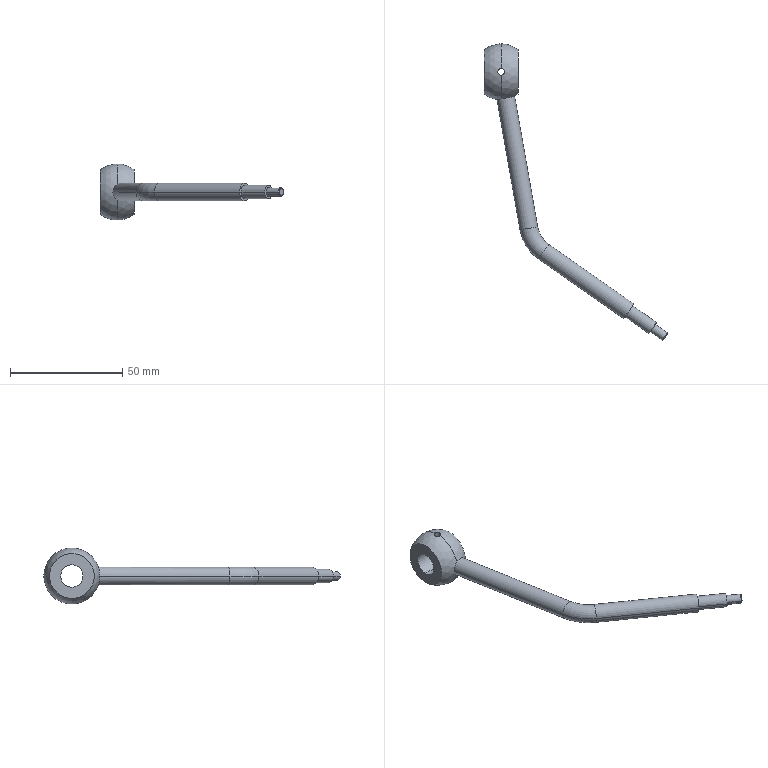Part | SolidWorks | features ICE 4, Revolution 1, StudWizard 1, Sweep 1, SweepCut 1 | 1 solid | 25 faces | box 81.686 x 132.115 x 24.819 mm | volume 11563 mm3 | cylinder 14 | plane 5 | torus 2 | cone 2 | sphere 2 | commonest cylinder face diameters 3 x4 8 x4 4 x2 6 x2 10 x2
STEP:
#1=CARTESIAN_POINT('',(8.368,-70.49,0.));
#2=VERTEX_POINT('',#1);
#3=CARTESIAN_POINT('',(16.246,-69.101,0.));
#4=VERTEX_POINT('',#3);
#5=CARTESIAN_POINT('',(12.307,-69.796,0.));
#6=DIRECTION('',(-0.1736,0.9848,0.));
#7=DIRECTION('',(-0.9848,-0.1736,0.));
#8=AXIS2_PLACEMENT_3D('',#5,#6,#7);
#9=CIRCLE('',#8,4.);
#10=EDGE_CURVE('',#2,#4,#9,.T.);
#11=ORIENTED_EDGE('',*,*,#10,.F.);
#12=CARTESIAN_POINT('',(16.592,-83.401,0.));
#13=VERTEX_POINT('',#12);
#14=CARTESIAN_POINT('',(28.064,-67.017,0.));
#15=DIRECTION('',(0.,0.,1.));
#16=DIRECTION('',(1.,0.,0.));
#17=AXIS2_PLACEMENT_3D('',#14,#15,#16);
#18=CIRCLE('',#17,20.);
#19=EDGE_CURVE('',#2,#13,#18,.T.);
#20=ORIENTED_EDGE('',*,*,#19,.T.);
#21=CARTESIAN_POINT('',(21.181,-76.847,0.));
#22=VERTEX_POINT('',#21);
#23=CARTESIAN_POINT('',(18.887,-80.124,0.));
#24=DIRECTION('',(-0.8192,0.5736,0.));
#25=DIRECTION('',(-0.5736,-0.8192,0.));
#26=AXIS2_PLACEMENT_3D('',#23,#24,#25);
#27=CIRCLE('',#26,4.);
#28=EDGE_CURVE('',#13,#22,#27,.T.);
#29=ORIENTED_EDGE('',*,*,#28,.T.);
#30=CARTESIAN_POINT('',(28.064,-67.017,0.));
#31=DIRECTION('',(0.,0.,1.));
#32=DIRECTION('',(1.,0.,0.));
#33=AXIS2_PLACEMENT_3D('',#30,#31,#32);
#34=CIRCLE('',#33,12.);
#35=EDGE_CURVE('',#4,#22,#34,.T.);
#36=ORIENTED_EDGE('',*,*,#35,.F.);
#37=EDGE_LOOP('',(#11,#20,#29,#36));
#38=FACE_OUTER_BOUND('',#37,.T.);
#39=CARTESIAN_POINT('',(28.064,-67.017,0.));
#40=DIRECTION('',(0.,0.,1.));
#41=DIRECTION('',(1.,0.,0.));
#42=AXIS2_PLACEMENT_3D('',#39,#40,#41);
#43=TOROIDAL_SURFACE('',#42,16.,4.);
#44=ADVANCED_FACE('',(#38),#43,.T.);
#45=CARTESIAN_POINT('',(1.5,0.,-5.));
#46=VERTEX_POINT('',#45);
#47=CARTESIAN_POINT('',(-1.5,0.,-5.));
#48=VERTEX_POINT('',#47);
#49=CARTESIAN_POINT('',(1.5,0.,-5.));
#50=CARTESIAN_POINT('',(1.5,-0.1965,-5.));
#51=CARTESIAN_POINT('',(1.46,-0.3949,-4.988));
#52=CARTESIAN_POINT('',(1.348,-0.6661,-4.956));
#53=CARTESIAN_POINT('',(1.3,-0.7539,-4.944));
#54=CARTESIAN_POINT('',(1.192,-0.9162,-4.916));
#55=CARTESIAN_POINT('',(1.13,-0.9913,-4.901));
#56=CARTESIAN_POINT('',(0.9224,-1.199,-4.856));
#57=CARTESIAN_POINT('',(0.7589,-1.309,-4.826));
#58=CARTESIAN_POINT('',(0.4847,-1.423,-4.793));
#59=CARTESIAN_POINT('',(0.3909,-1.451,-4.785));
#60=CARTESIAN_POINT('',(0.1987,-1.49,-4.773));
#61=CARTESIAN_POINT('',(0.09898,-1.5,-4.77));
#62=CARTESIAN_POINT('',(-0.09875,-1.5,-4.77));
#63=CARTESIAN_POINT('',(-0.1965,-1.49,-4.773));
#64=CARTESIAN_POINT('',(-0.3898,-1.452,-4.785));
#65=CARTESIAN_POINT('',(-0.4854,-1.423,-4.793));
#66=CARTESIAN_POINT('',(-0.7564,-1.31,-4.826));
#67=CARTESIAN_POINT('',(-0.9227,-1.199,-4.856));
#68=CARTESIAN_POINT('',(-1.129,-0.9924,-4.901));
#69=CARTESIAN_POINT('',(-1.192,-0.9159,-4.916));
#70=CARTESIAN_POINT('',(-1.301,-0.7533,-4.944));
#71=CARTESIAN_POINT('',(-1.347,-0.6674,-4.956));
#72=CARTESIAN_POINT('',(-1.422,-0.4865,-4.977));
#73=CARTESIAN_POINT('',(-1.452,-0.3907,-4.986));
#74=CARTESIAN_POINT('',(-1.49,-0.1978,-4.997));
#75=CARTESIAN_POINT('',(-1.5,-0.0997,-5.));
#76=CARTESIAN_POINT('',(-1.5,0.,-5.));
#77=B_SPLINE_CURVE_WITH_KNOTS('',3,(#49,#50,#51,#52,#53,#54,#55,#56,#57,#58,#59,#60,#61,#62,#63,#64,#65,#66,#67,#68,#69,#70,#71,#72,#73,#74,#75,#76),.UNSPECIFIED.,.F.,.F.,(4,2,2,2,2,2,2,2,2,2,2,2,2,4),(0.004717,0.005306,0.005601,0.005896,0.006485,0.00678,0.007075,0.00737,0.007664,0.008254,0.008549,0.008843,0.009138,0.009433),.UNSPECIFIED.);
#78=EDGE_CURVE('',#46,#48,#77,.T.);
#79=ORIENTED_EDGE('',*,*,#78,.F.);
#80=CARTESIAN_POINT('',(1.5,0.,-12.41));
#81=VERTEX_POINT('',#80);
#82=CARTESIAN_POINT('',(1.5,0.,14.908));
#83=DIRECTION('',(0.,0.,-1.));
#84=VECTOR('',#83,1000.);
#85=LINE('',#82,#84);
#86=EDGE_CURVE('',#46,#81,#85,.T.);
#87=ORIENTED_EDGE('',*,*,#86,.T.);
#88=CARTESIAN_POINT('',(0.,-1.5,-12.41));
#89=VERTEX_POINT('',#88);
#90=CARTESIAN_POINT('',(0.,0.,-12.41));
#91=DIRECTION('',(0.,0.,-1.));
#92=DIRECTION('',(1.,0.,0.));
#93=AXIS2_PLACEMENT_3D('',#90,#91,#92);
#94=CIRCLE('',#93,1.5);
#95=EDGE_CURVE('',#81,#89,#94,.T.);
#96=ORIENTED_EDGE('',*,*,#95,.T.);
#97=CARTESIAN_POINT('',(-1.5,0.,-12.41));
#98=VERTEX_POINT('',#97);
#99=CARTESIAN_POINT('',(0.,0.,-12.41));
#100=DIRECTION('',(0.,0.,-1.));
#101=DIRECTION('',(1.,0.,0.));
#102=AXIS2_PLACEMENT_3D('',#99,#100,#101);
#103=CIRCLE('',#102,1.5);
#104=EDGE_CURVE('',#89,#98,#103,.T.);
#105=ORIENTED_EDGE('',*,*,#104,.T.);
#106=CARTESIAN_POINT('',(-1.5,0.,14.908));
#107=DIRECTION('',(0.,0.,-1.));
#108=VECTOR('',#107,1000.);
#109=LINE('',#106,#108);
#110=EDGE_CURVE('',#48,#98,#109,.T.);
#111=ORIENTED_EDGE('',*,*,#110,.F.);
#112=EDGE_LOOP('',(#79,#87,#96,#105,#111));
#113=FACE_OUTER_BOUND('',#112,.T.);
#114=CARTESIAN_POINT('',(0.,0.,14.908));
#115=DIRECTION('',(0.,0.,-1.));
#116=DIRECTION('',(-1.,0.,0.));
#117=AXIS2_PLACEMENT_3D('',#114,#115,#116);
#118=CYLINDRICAL_SURFACE('',#117,1.5);
#119=ADVANCED_FACE('',(#113),#118,.F.);
#120=CARTESIAN_POINT('',(0.,-1.5,12.41));
#121=VERTEX_POINT('',#120);
#122=CARTESIAN_POINT('',(1.5,0.,12.41));
#123=VERTEX_POINT('',#122);
#124=CARTESIAN_POINT('',(0.,0.,12.41));
#125=DIRECTION('',(0.,0.,1.));
#126=DIRECTION('',(-1.,0.,0.));
#127=AXIS2_PLACEMENT_3D('',#124,#125,#126);
#128=CIRCLE('',#127,1.5);
#129=EDGE_CURVE('',#121,#123,#128,.T.);
#130=ORIENTED_EDGE('',*,*,#129,.T.);
#131=CARTESIAN_POINT('',(1.5,0.,5.));
#132=VERTEX_POINT('',#131);
#133=CARTESIAN_POINT('',(1.5,0.,14.908));
#134=DIRECTION('',(0.,0.,-1.));
#135=VECTOR('',#134,1000.);
#136=LINE('',#133,#135);
#137=EDGE_CURVE('',#123,#132,#136,.T.);
#138=ORIENTED_EDGE('',*,*,#137,.T.);
#139=CARTESIAN_POINT('',(-1.5,0.,5.));
#140=VERTEX_POINT('',#139);
#141=CARTESIAN_POINT('',(-1.5,0.,5.));
#142=CARTESIAN_POINT('',(-1.5,-0.09973,5.));
#143=CARTESIAN_POINT('',(-1.49,-0.1977,4.997));
#144=CARTESIAN_POINT('',(-1.452,-0.3902,4.986));
#145=CARTESIAN_POINT('',(-1.423,-0.4858,4.977));
#146=CARTESIAN_POINT('',(-1.347,-0.6672,4.956));
#147=CARTESIAN_POINT('',(-1.301,-0.7532,4.944));
#148=CARTESIAN_POINT('',(-1.192,-0.9158,4.916));
#149=CARTESIAN_POINT('',(-1.129,-0.9923,4.901));
#150=CARTESIAN_POINT('',(-0.9227,-1.199,4.856));
#151=CARTESIAN_POINT('',(-0.7563,-1.31,4.826));
#152=CARTESIAN_POINT('',(-0.3958,-1.46,4.783));
#153=CARTESIAN_POINT('',(-0.1976,-1.5,4.77));
#154=CARTESIAN_POINT('',(0.09779,-1.5,4.77));
#155=CARTESIAN_POINT('',(0.1978,-1.49,4.773));
#156=CARTESIAN_POINT('',(0.3907,-1.452,4.785));
#157=CARTESIAN_POINT('',(0.4845,-1.423,4.793));
#158=CARTESIAN_POINT('',(0.758,-1.309,4.826));
#159=CARTESIAN_POINT('',(0.9226,-1.199,4.856));
#160=CARTESIAN_POINT('',(1.13,-0.9911,4.901));
#161=CARTESIAN_POINT('',(1.192,-0.9159,4.916));
#162=CARTESIAN_POINT('',(1.3,-0.7538,4.944));
#163=CARTESIAN_POINT('',(1.348,-0.666,4.956));
#164=CARTESIAN_POINT('',(1.423,-0.4851,4.977));
#165=CARTESIAN_POINT('',(1.451,-0.3916,4.986));
#166=CARTESIAN_POINT('',(1.49,-0.1978,4.997));
#167=CARTESIAN_POINT('',(1.5,-0.09827,5.));
#168=CARTESIAN_POINT('',(1.5,0.,5.));
#169=B_SPLINE_CURVE_WITH_KNOTS('',3,(#141,#142,#143,#144,#145,#146,#147,#148,#149,#150,#151,#152,#153,#154,#155,#156,#157,#158,#159,#160,#161,#162,#163,#164,#165,#166,#167,#168),.UNSPECIFIED.,.F.,.F.,(4,2,2,2,2,2,2,2,2,2,2,2,2,4),(0.,0.0002948,0.0005896,0.0008844,0.001179,0.001769,0.002359,0.002653,0.002948,0.003538,0.003833,0.004127,0.004422,0.004717),.UNSPECIFIED.);
#170=EDGE_CURVE('',#140,#132,#169,.T.);
#171=ORIENTED_EDGE('',*,*,#170,.F.);
#172=CARTESIAN_POINT('',(-1.5,0.,12.41));
#173=VERTEX_POINT('',#172);
#174=CARTESIAN_POINT('',(-1.5,0.,14.908));
#175=DIRECTION('',(0.,0.,-1.));
#176=VECTOR('',#175,1000.);
#177=LINE('',#174,#176);
#178=EDGE_CURVE('',#173,#140,#177,.T.);
#179=ORIENTED_EDGE('',*,*,#178,.F.);
#180=CARTESIAN_POINT('',(0.,0.,12.41));
#181=DIRECTION('',(0.,0.,1.));
#182=DIRECTION('',(-1.,0.,0.));
#183=AXIS2_PLACEMENT_3D('',#180,#181,#182);
#184=CIRCLE('',#183,1.5);
#185=EDGE_CURVE('',#173,#121,#184,.T.);
#186=ORIENTED_EDGE('',*,*,#185,.T.);
#187=EDGE_LOOP('',(#130,#138,#171,#179,#186));
#188=FACE_OUTER_BOUND('',#187,.T.);
#189=CARTESIAN_POINT('',(0.,0.,14.908));
#190=DIRECTION('',(0.,0.,-1.));
#191=DIRECTION('',(-1.,0.,0.));
#192=AXIS2_PLACEMENT_3D('',#189,#190,#191);
#193=CYLINDRICAL_SURFACE('',#192,1.5);
#194=ADVANCED_FACE('',(#188),#193,.F.);
#195=CARTESIAN_POINT('',(-7.5,0.,5.));
#196=VERTEX_POINT('',#195);
#197=CARTESIAN_POINT('',(-7.5,0.,-5.));
#198=VERTEX_POINT('',#197);
#199=CARTESIAN_POINT('',(-7.5,0.,0.));
#200=DIRECTION('',(1.,0.,0.));
#201=DIRECTION('',(0.,0.,-1.));
#202=AXIS2_PLACEMENT_3D('',#199,#200,#201);
#203=CIRCLE('',#202,5.);
#204=EDGE_CURVE('',#196,#198,#203,.T.);
#205=ORIENTED_EDGE('',*,*,#204,.F.);
#206=CARTESIAN_POINT('',(-7.5,0.,5.));
#207=DIRECTION('',(1.,0.,0.));
#208=VECTOR('',#207,1000.);
#209=LINE('',#206,#208);
#210=EDGE_CURVE('',#196,#140,#209,.T.);
#211=ORIENTED_EDGE('',*,*,#210,.T.);
#212=ORIENTED_EDGE('',*,*,#170,.T.);
#213=CARTESIAN_POINT('',(7.5,0.,5.));
#214=VERTEX_POINT('',#213);
#215=CARTESIAN_POINT('',(-7.5,0.,5.));
#216=DIRECTION('',(1.,0.,0.));
#217=VECTOR('',#216,1000.);
#218=LINE('',#215,#217);
#219=EDGE_CURVE('',#132,#214,#218,.T.);
#220=ORIENTED_EDGE('',*,*,#219,.T.);
#221=CARTESIAN_POINT('',(7.5,0.,-5.));
#222=VERTEX_POINT('',#221);
#223=CARTESIAN_POINT('',(7.5,0.,0.));
#224=DIRECTION('',(-1.,0.,0.));
#225=DIRECTION('',(0.,0.,1.));
#226=AXIS2_PLACEMENT_3D('',#223,#224,#225);
#227=CIRCLE('',#226,5.);
#228=EDGE_CURVE('',#222,#214,#227,.T.);
#229=ORIENTED_EDGE('',*,*,#228,.F.);
#230=CARTESIAN_POINT('',(-7.5,0.,-5.));
#231=DIRECTION('',(1.,0.,0.));
#232=VECTOR('',#231,1000.);
#233=LINE('',#230,#232);
#234=EDGE_CURVE('',#46,#222,#233,.T.);
#235=ORIENTED_EDGE('',*,*,#234,.F.);
#236=ORIENTED_EDGE('',*,*,#78,.T.);
#237=CARTESIAN_POINT('',(-7.5,0.,-5.));
#238=DIRECTION('',(1.,0.,0.));
#239=VECTOR('',#238,1000.);
#240=LINE('',#237,#239);
#241=EDGE_CURVE('',#198,#48,#240,.T.);
#242=ORIENTED_EDGE('',*,*,#241,.F.);
#243=EDGE_LOOP('',(#205,#211,#212,#220,#229,#235,#236,#242));
#244=FACE_OUTER_BOUND('',#243,.T.);
#245=CARTESIAN_POINT('',(-7.5,0.,0.));
#246=DIRECTION('',(1.,0.,0.));
#247=DIRECTION('',(0.,0.,-1.));
#248=AXIS2_PLACEMENT_3D('',#245,#246,#247);
#249=CYLINDRICAL_SURFACE('',#248,5.);
#250=ADVANCED_FACE('',(#244),#249,.F.);
#251=CARTESIAN_POINT('',(72.326,-119.522,0.));
#252=VERTEX_POINT('',#251);
#253=CARTESIAN_POINT('',(74.186,-116.866,0.));
#254=VERTEX_POINT('',#253);
#255=CARTESIAN_POINT('',(73.256,-118.194,0.));
#256=DIRECTION('',(-0.8192,0.5736,0.));
#257=DIRECTION('',(-0.5736,-0.8192,0.));
#258=AXIS2_PLACEMENT_3D('',#255,#256,#257);
#259=CIRCLE('',#258,1.621);
#260=EDGE_CURVE('',#252,#254,#259,.T.);
#261=ORIENTED_EDGE('',*,*,#260,.T.);
#262=CARTESIAN_POINT('',(74.093,-116.338,0.));
#263=VERTEX_POINT('',#262);
#264=CARTESIAN_POINT('',(74.186,-116.866,0.));
#265=DIRECTION('',(-0.1736,0.9848,0.));
#266=VECTOR('',#265,1000.);
#267=LINE('',#264,#266);
#268=EDGE_CURVE('',#254,#263,#267,.T.);
#269=ORIENTED_EDGE('',*,*,#268,.T.);
#270=CARTESIAN_POINT('',(71.798,-119.615,0.));
#271=VERTEX_POINT('',#270);
#272=CARTESIAN_POINT('',(72.945,-117.976,0.));
#273=DIRECTION('',(-0.8192,0.5736,0.));
#274=DIRECTION('',(-0.5736,-0.8192,0.));
#275=AXIS2_PLACEMENT_3D('',#272,#273,#274);
#276=CIRCLE('',#275,2.);
#277=EDGE_CURVE('',#271,#263,#276,.T.);
#278=ORIENTED_EDGE('',*,*,#277,.F.);
#279=CARTESIAN_POINT('',(72.326,-119.522,0.));
#280=DIRECTION('',(-0.9848,-0.1736,0.));
#281=VECTOR('',#280,1000.);
#282=LINE('',#279,#281);
#283=EDGE_CURVE('',#252,#271,#282,.T.);
#284=ORIENTED_EDGE('',*,*,#283,.F.);
#285=EDGE_LOOP('',(#261,#269,#278,#284));
#286=FACE_OUTER_BOUND('',#285,.T.);
#287=CARTESIAN_POINT('',(73.256,-118.194,0.));
#288=DIRECTION('',(-0.8192,0.5736,0.));
#289=DIRECTION('',(-0.5736,-0.8192,0.));
#290=AXIS2_PLACEMENT_3D('',#287,#288,#289);
#291=CONICAL_SURFACE('',#290,1.621,0.7854);
#292=ADVANCED_FACE('',(#286),#291,.T.);
#293=ORIENTED_EDGE('',*,*,#277,.T.);
#294=CARTESIAN_POINT('',(68.669,-112.54,0.));
#295=VERTEX_POINT('',#294);
#296=CARTESIAN_POINT('',(74.403,-116.555,0.));
#297=DIRECTION('',(-0.8192,0.5736,0.));
#298=VECTOR('',#297,1000.);
#299=LINE('',#296,#298);
#300=EDGE_CURVE('',#263,#295,#299,.T.);
#301=ORIENTED_EDGE('',*,*,#300,.T.);
#302=CARTESIAN_POINT('',(66.375,-115.817,0.));
#303=VERTEX_POINT('',#302);
#304=CARTESIAN_POINT('',(67.522,-114.179,0.));
#305=DIRECTION('',(0.8192,-0.5736,0.));
#306=DIRECTION('',(0.5736,0.8192,0.));
#307=AXIS2_PLACEMENT_3D('',#304,#305,#306);
#308=CIRCLE('',#307,2.);
#309=EDGE_CURVE('',#295,#303,#308,.T.);
#310=ORIENTED_EDGE('',*,*,#309,.T.);
#311=CARTESIAN_POINT('',(72.109,-119.832,0.));
#312=DIRECTION('',(-0.8192,0.5736,0.));
#313=VECTOR('',#312,1000.);
#314=LINE('',#311,#313);
#315=EDGE_CURVE('',#271,#303,#314,.T.);
#316=ORIENTED_EDGE('',*,*,#315,.F.);
#317=EDGE_LOOP('',(#293,#301,#310,#316));
#318=FACE_OUTER_BOUND('',#317,.T.);
#319=CARTESIAN_POINT('',(73.256,-118.194,0.));
#320=DIRECTION('',(-0.8192,0.5736,0.));
#321=DIRECTION('',(-0.5736,-0.8192,0.));
#322=AXIS2_PLACEMENT_3D('',#319,#320,#321);
#323=CYLINDRICAL_SURFACE('',#322,2.);
#324=ADVANCED_FACE('',(#318),#323,.T.);
#325=CARTESIAN_POINT('',(69.242,-111.721,0.));
#326=VERTEX_POINT('',#325);
#327=CARTESIAN_POINT('',(65.801,-116.636,0.));
#328=VERTEX_POINT('',#327);
#329=CARTESIAN_POINT('',(67.522,-114.179,0.));
#330=DIRECTION('',(0.8192,-0.5736,0.));
#331=DIRECTION('',(0.5736,0.8192,0.));
#332=AXIS2_PLACEMENT_3D('',#329,#330,#331);
#333=CIRCLE('',#332,3.);
#334=EDGE_CURVE('',#326,#328,#333,.T.);
#335=ORIENTED_EDGE('',*,*,#334,.F.);
#336=CARTESIAN_POINT('',(58.594,-104.265,0.));
#337=VERTEX_POINT('',#336);
#338=CARTESIAN_POINT('',(69.242,-111.721,0.));
#339=DIRECTION('',(-0.8192,0.5736,0.));
#340=VECTOR('',#339,1000.);
#341=LINE('',#338,#340);
#342=EDGE_CURVE('',#326,#337,#341,.T.);
#343=ORIENTED_EDGE('',*,*,#342,.T.);
#344=CARTESIAN_POINT('',(55.152,-109.18,0.));
#345=VERTEX_POINT('',#344);
#346=CARTESIAN_POINT('',(56.873,-106.722,0.));
#347=DIRECTION('',(0.8192,-0.5736,0.));
#348=DIRECTION('',(0.5736,0.8192,0.));
#349=AXIS2_PLACEMENT_3D('',#346,#347,#348);
#350=CIRCLE('',#349,3.);
#351=EDGE_CURVE('',#337,#345,#350,.T.);
#352=ORIENTED_EDGE('',*,*,#351,.T.);
#353=CARTESIAN_POINT('',(65.801,-116.636,0.));
#354=DIRECTION('',(-0.8192,0.5736,0.));
#355=VECTOR('',#354,1000.);
#356=LINE('',#353,#355);
#357=EDGE_CURVE('',#328,#345,#356,.T.);
#358=ORIENTED_EDGE('',*,*,#357,.F.);
#359=EDGE_LOOP('',(#335,#343,#352,#358));
#360=FACE_OUTER_BOUND('',#359,.T.);
#361=CARTESIAN_POINT('',(67.522,-114.179,0.));
#362=DIRECTION('',(-0.8192,0.5736,0.));
#363=DIRECTION('',(-0.5736,-0.8192,0.));
#364=AXIS2_PLACEMENT_3D('',#361,#362,#363);
#365=CYLINDRICAL_SURFACE('',#364,3.);
#366=ADVANCED_FACE('',(#360),#365,.T.);
#367=CARTESIAN_POINT('',(-7.5,0.,-10.));
#368=VERTEX_POINT('',#367);
#369=CARTESIAN_POINT('',(-7.5,0.,10.));
#370=VERTEX_POINT('',#369);
#371=CARTESIAN_POINT('',(-7.5,0.,0.));
#372=DIRECTION('',(-1.,0.,0.));
#373=DIRECTION('',(0.,0.,-1.));
#374=AXIS2_PLACEMENT_3D('',#371,#372,#373);
#375=CIRCLE('',#374,10.);
#376=EDGE_CURVE('',#368,#370,#375,.T.);
#377=ORIENTED_EDGE('',*,*,#376,.F.);
#378=CARTESIAN_POINT('',(-7.5,0.,0.));
#379=DIRECTION('',(-1.,0.,0.));
#380=DIRECTION('',(0.,0.,-1.));
#381=AXIS2_PLACEMENT_3D('',#378,#379,#380);
#382=CIRCLE('',#381,10.);
#383=EDGE_CURVE('',#370,#368,#382,.T.);
#384=ORIENTED_EDGE('',*,*,#383,.F.);
#385=EDGE_LOOP('',(#377,#384));
#386=FACE_BOUND('',#385,.T.);
#387=CARTESIAN_POINT('',(-1.883,-12.357,0.));
#388=VERTEX_POINT('',#387);
#389=CARTESIAN_POINT('',(0.,-12.025,3.412));
#390=VERTEX_POINT('',#389);
#391=CARTESIAN_POINT('',(2.056,-11.663,0.));
#392=DIRECTION('',(-0.1736,0.9848,0.));
#393=DIRECTION('',(-0.9848,-0.1736,0.));
#394=AXIS2_PLACEMENT_3D('',#391,#392,#393);
#395=CIRCLE('',#394,4.);
#396=EDGE_CURVE('',#388,#390,#395,.T.);
#397=ORIENTED_EDGE('',*,*,#396,.T.);
#398=CARTESIAN_POINT('',(0.,0.,0.));
#399=DIRECTION('',(-1.,0.,0.));
#400=DIRECTION('',(0.,0.,1.));
#401=AXIS2_PLACEMENT_3D('',#398,#399,#400);
#402=CIRCLE('',#401,12.5);
#403=EDGE_CURVE('',#390,#121,#402,.T.);
#404=ORIENTED_EDGE('',*,*,#403,.T.);
#405=ORIENTED_EDGE('',*,*,#185,.F.);
#406=CARTESIAN_POINT('',(0.,1.5,12.41));
#407=VERTEX_POINT('',#406);
#408=CARTESIAN_POINT('',(0.,0.,12.41));
#409=DIRECTION('',(0.,0.,1.));
#410=DIRECTION('',(-1.,0.,0.));
#411=AXIS2_PLACEMENT_3D('',#408,#409,#410);
#412=CIRCLE('',#411,1.5);
#413=EDGE_CURVE('',#407,#173,#412,.T.);
#414=ORIENTED_EDGE('',*,*,#413,.F.);
#415=CARTESIAN_POINT('',(0.,12.5,0.));
#416=VERTEX_POINT('',#415);
#417=CARTESIAN_POINT('',(0.,0.,0.));
#418=DIRECTION('',(-1.,0.,0.));
#419=DIRECTION('',(0.,0.,1.));
#420=AXIS2_PLACEMENT_3D('',#417,#418,#419);
#421=CIRCLE('',#420,12.5);
#422=EDGE_CURVE('',#407,#416,#421,.T.);
#423=ORIENTED_EDGE('',*,*,#422,.T.);
#424=CARTESIAN_POINT('',(0.,1.5,-12.41));
#425=VERTEX_POINT('',#424);
#426=CARTESIAN_POINT('',(0.,0.,0.));
#427=DIRECTION('',(1.,0.,0.));
#428=DIRECTION('',(0.,0.,-1.));
#429=AXIS2_PLACEMENT_3D('',#426,#427,#428);
#430=CIRCLE('',#429,12.5);
#431=EDGE_CURVE('',#425,#416,#430,.T.);
#432=ORIENTED_EDGE('',*,*,#431,.F.);
#433=CARTESIAN_POINT('',(0.,0.,-12.41));
#434=DIRECTION('',(0.,0.,-1.));
#435=DIRECTION('',(1.,0.,0.));
#436=AXIS2_PLACEMENT_3D('',#433,#434,#435);
#437=CIRCLE('',#436,1.5);
#438=EDGE_CURVE('',#98,#425,#437,.T.);
#439=ORIENTED_EDGE('',*,*,#438,.F.);
#440=ORIENTED_EDGE('',*,*,#104,.F.);
#441=CARTESIAN_POINT('',(0.,-12.025,-3.412));
#442=VERTEX_POINT('',#441);
#443=CARTESIAN_POINT('',(0.,0.,0.));
#444=DIRECTION('',(1.,0.,0.));
#445=DIRECTION('',(0.,0.,-1.));
#446=AXIS2_PLACEMENT_3D('',#443,#444,#445);
#447=CIRCLE('',#446,12.5);
#448=EDGE_CURVE('',#442,#89,#447,.T.);
#449=ORIENTED_EDGE('',*,*,#448,.F.);
#450=CARTESIAN_POINT('',(2.056,-11.663,0.));
#451=DIRECTION('',(-0.1736,0.9848,0.));
#452=DIRECTION('',(-0.9848,-0.1736,0.));
#453=AXIS2_PLACEMENT_3D('',#450,#451,#452);
#454=CIRCLE('',#453,4.);
#455=EDGE_CURVE('',#442,#388,#454,.T.);
#456=ORIENTED_EDGE('',*,*,#455,.T.);
#457=EDGE_LOOP('',(#397,#404,#405,#414,#423,#432,#439,#440,#449,#456));
#458=FACE_OUTER_BOUND('',#457,.T.);
#459=CARTESIAN_POINT('',(0.,0.,0.));
#460=DIRECTION('',(-1.,0.,0.));
#461=DIRECTION('',(0.,0.,-1.));
#462=AXIS2_PLACEMENT_3D('',#459,#460,#461);
#463=SPHERICAL_SURFACE('',#462,12.5);
#464=ADVANCED_FACE('',(#386,#458),#463,.T.);
#465=ORIENTED_EDGE('',*,*,#28,.F.);
#466=CARTESIAN_POINT('',(54.578,-109.999,0.));
#467=VERTEX_POINT('',#466);
#468=CARTESIAN_POINT('',(16.592,-83.401,0.));
#469=DIRECTION('',(0.8192,-0.5736,0.));
#470=VECTOR('',#469,1000.);
#471=LINE('',#468,#470);
#472=EDGE_CURVE('',#13,#467,#471,.T.);
#473=ORIENTED_EDGE('',*,*,#472,.T.);
#474=CARTESIAN_POINT('',(59.167,-103.446,0.));
#475=VERTEX_POINT('',#474);
#476=CARTESIAN_POINT('',(56.873,-106.722,0.));
#477=DIRECTION('',(-0.8192,0.5736,0.));
#478=DIRECTION('',(-0.5736,-0.8192,0.));
#479=AXIS2_PLACEMENT_3D('',#476,#477,#478);
#480=CIRCLE('',#479,4.);
#481=EDGE_CURVE('',#467,#475,#480,.T.);
#482=ORIENTED_EDGE('',*,*,#481,.T.);
#483=CARTESIAN_POINT('',(21.181,-76.847,0.));
#484=DIRECTION('',(0.8192,-0.5736,0.));
#485=VECTOR('',#484,1000.);
#486=LINE('',#483,#485);
#487=EDGE_CURVE('',#22,#475,#486,.T.);
#488=ORIENTED_EDGE('',*,*,#487,.F.);
#489=EDGE_LOOP('',(#465,#473,#482,#488));
#490=FACE_OUTER_BOUND('',#489,.T.);
#491=CARTESIAN_POINT('',(18.887,-80.124,0.));
#492=DIRECTION('',(0.8192,-0.5736,0.));
#493=DIRECTION('',(0.5736,0.8192,0.));
#494=AXIS2_PLACEMENT_3D('',#491,#492,#493);
#495=CYLINDRICAL_SURFACE('',#494,4.);
#496=ADVANCED_FACE('',(#490),#495,.T.);
#497=ORIENTED_EDGE('',*,*,#396,.F.);
#498=CARTESIAN_POINT('',(-3.939,-0.6946,0.));
#499=DIRECTION('',(0.1736,-0.9848,0.));
#500=VECTOR('',#499,1000.);
#501=LINE('',#498,#500);
#502=EDGE_CURVE('',#388,#2,#501,.T.);
#503=ORIENTED_EDGE('',*,*,#502,.T.);
#504=ORIENTED_EDGE('',*,*,#10,.T.);
#505=CARTESIAN_POINT('',(5.996,-10.968,0.));
#506=VERTEX_POINT('',#505);
#507=CARTESIAN_POINT('',(3.939,0.6946,0.));
#508=DIRECTION('',(0.1736,-0.9848,0.));
#509=VECTOR('',#508,1000.);
#510=LINE('',#507,#509);
#511=EDGE_CURVE('',#506,#4,#510,.T.);
#512=ORIENTED_EDGE('',*,*,#511,.F.);
#513=CARTESIAN_POINT('',(2.056,-11.663,0.));
#514=DIRECTION('',(-0.1736,0.9848,0.));
#515=DIRECTION('',(-0.9848,-0.1736,0.));
#516=AXIS2_PLACEMENT_3D('',#513,#514,#515);
#517=CIRCLE('',#516,4.);
#518=EDGE_CURVE('',#390,#506,#517,.T.);
#519=ORIENTED_EDGE('',*,*,#518,.F.);
#520=EDGE_LOOP('',(#497,#503,#504,#512,#519));
#521=FACE_OUTER_BOUND('',#520,.T.);
#522=CARTESIAN_POINT('',(0.,0.,0.));
#523=DIRECTION('',(0.1736,-0.9848,0.));
#524=DIRECTION('',(0.9848,0.1736,0.));
#525=AXIS2_PLACEMENT_3D('',#522,#523,#524);
#526=CYLINDRICAL_SURFACE('',#525,4.);
#527=ADVANCED_FACE('',(#521),#526,.T.);
#528=ORIENTED_EDGE('',*,*,#472,.F.);
#529=CARTESIAN_POINT('',(18.887,-80.124,0.));
#530=DIRECTION('',(-0.8192,0.5736,0.));
#531=DIRECTION('',(-0.5736,-0.8192,0.));
#532=AXIS2_PLACEMENT_3D('',#529,#530,#531);
#533=CIRCLE('',#532,4.);
#534=EDGE_CURVE('',#22,#13,#533,.T.);
#535=ORIENTED_EDGE('',*,*,#534,.F.);
#536=ORIENTED_EDGE('',*,*,#487,.T.);
#537=CARTESIAN_POINT('',(56.873,-106.722,0.));
#538=DIRECTION('',(-0.8192,0.5736,0.));
#539=DIRECTION('',(-0.5736,-0.8192,0.));
#540=AXIS2_PLACEMENT_3D('',#537,#538,#539);
#541=CIRCLE('',#540,4.);
#542=EDGE_CURVE('',#475,#467,#541,.T.);
#543=ORIENTED_EDGE('',*,*,#542,.T.);
#544=EDGE_LOOP('',(#528,#535,#536,#543));
#545=FACE_OUTER_BOUND('',#544,.T.);
#546=CARTESIAN_POINT('',(18.887,-80.124,0.));
#547=DIRECTION('',(0.8192,-0.5736,0.));
#548=DIRECTION('',(0.5736,0.8192,0.));
#549=AXIS2_PLACEMENT_3D('',#546,#547,#548);
#550=CYLINDRICAL_SURFACE('',#549,4.);
#551=ADVANCED_FACE('',(#545),#550,.T.);
#552=ORIENTED_EDGE('',*,*,#19,.F.);
#553=CARTESIAN_POINT('',(12.307,-69.796,0.));
#554=DIRECTION('',(-0.1736,0.9848,0.));
#555=DIRECTION('',(-0.9848,-0.1736,0.));
#556=AXIS2_PLACEMENT_3D('',#553,#554,#555);
#557=CIRCLE('',#556,4.);
#558=EDGE_CURVE('',#4,#2,#557,.T.);
#559=ORIENTED_EDGE('',*,*,#558,.F.);
#560=ORIENTED_EDGE('',*,*,#35,.T.);
#561=ORIENTED_EDGE('',*,*,#534,.T.);
#562=EDGE_LOOP('',(#552,#559,#560,#561));
#563=FACE_OUTER_BOUND('',#562,.T.);
#564=CARTESIAN_POINT('',(28.064,-67.017,0.));
#565=DIRECTION('',(0.,0.,1.));
#566=DIRECTION('',(1.,0.,0.));
#567=AXIS2_PLACEMENT_3D('',#564,#565,#566);
#568=TOROIDAL_SURFACE('',#567,16.,4.);
#569=ADVANCED_FACE('',(#563),#568,.T.);
#570=ORIENTED_EDGE('',*,*,#502,.F.);
#571=ORIENTED_EDGE('',*,*,#455,.F.);
#572=CARTESIAN_POINT('',(2.056,-11.663,0.));
#573=DIRECTION('',(-0.1736,0.9848,0.));
#574=DIRECTION('',(-0.9848,-0.1736,0.));
#575=AXIS2_PLACEMENT_3D('',#572,#573,#574);
#576=CIRCLE('',#575,4.);
#577=EDGE_CURVE('',#506,#442,#576,.T.);
#578=ORIENTED_EDGE('',*,*,#577,.F.);
#579=ORIENTED_EDGE('',*,*,#511,.T.);
#580=ORIENTED_EDGE('',*,*,#558,.T.);
#581=EDGE_LOOP('',(#570,#571,#578,#579,#580));
#582=FACE_OUTER_BOUND('',#581,.T.);
#583=CARTESIAN_POINT('',(0.,0.,0.));
#584=DIRECTION('',(0.1736,-0.9848,0.));
#585=DIRECTION('',(0.9848,0.1736,0.));
#586=AXIS2_PLACEMENT_3D('',#583,#584,#585);
#587=CYLINDRICAL_SURFACE('',#586,4.);
#588=ADVANCED_FACE('',(#582),#587,.T.);
#589=CARTESIAN_POINT('',(56.873,-106.722,0.));
#590=DIRECTION('',(0.8192,-0.5736,0.));
#591=DIRECTION('',(0.5736,0.8192,0.));
#592=AXIS2_PLACEMENT_3D('',#589,#590,#591);
#593=CIRCLE('',#592,3.);
#594=EDGE_CURVE('',#345,#337,#593,.T.);
#595=ORIENTED_EDGE('',*,*,#594,.F.);
#596=ORIENTED_EDGE('',*,*,#351,.F.);
#597=EDGE_LOOP('',(#595,#596));
#598=FACE_BOUND('',#597,.T.);
#599=ORIENTED_EDGE('',*,*,#542,.F.);
#600=ORIENTED_EDGE('',*,*,#481,.F.);
#601=EDGE_LOOP('',(#599,#600));
#602=FACE_OUTER_BOUND('',#601,.T.);
#603=CARTESIAN_POINT('',(56.873,-106.722,0.));
#604=DIRECTION('',(-0.8192,0.5736,0.));
#605=DIRECTION('',(-0.5736,-0.8192,0.));
#606=AXIS2_PLACEMENT_3D('',#603,#604,#605);
#607=PLANE('',#606);
#608=ADVANCED_FACE('',(#598,#602),#607,.F.);
#609=ORIENTED_EDGE('',*,*,#403,.F.);
#610=ORIENTED_EDGE('',*,*,#518,.T.);
#611=ORIENTED_EDGE('',*,*,#577,.T.);
#612=ORIENTED_EDGE('',*,*,#448,.T.);
#613=ORIENTED_EDGE('',*,*,#95,.F.);
#614=CARTESIAN_POINT('',(0.,0.,-12.41));
#615=DIRECTION('',(0.,0.,-1.));
#616=DIRECTION('',(1.,0.,0.));
#617=AXIS2_PLACEMENT_3D('',#614,#615,#616);
#618=CIRCLE('',#617,1.5);
#619=EDGE_CURVE('',#425,#81,#618,.T.);
#620=ORIENTED_EDGE('',*,*,#619,.F.);
#621=ORIENTED_EDGE('',*,*,#431,.T.);
#622=ORIENTED_EDGE('',*,*,#422,.F.);
#623=CARTESIAN_POINT('',(0.,0.,12.41));
#624=DIRECTION('',(0.,0.,1.));
#625=DIRECTION('',(-1.,0.,0.));
#626=AXIS2_PLACEMENT_3D('',#623,#624,#625);
#627=CIRCLE('',#626,1.5);
#628=EDGE_CURVE('',#123,#407,#627,.T.);
#629=ORIENTED_EDGE('',*,*,#628,.F.);
#630=ORIENTED_EDGE('',*,*,#129,.F.);
#631=EDGE_LOOP('',(#609,#610,#611,#612,#613,#620,#621,#622,#629,#630));
#632=FACE_OUTER_BOUND('',#631,.T.);
#633=CARTESIAN_POINT('',(7.5,0.,10.));
#634=VERTEX_POINT('',#633);
#635=CARTESIAN_POINT('',(7.5,0.,-10.));
#636=VERTEX_POINT('',#635);
#637=CARTESIAN_POINT('',(7.5,0.,0.));
#638=DIRECTION('',(1.,0.,0.));
#639=DIRECTION('',(0.,0.,1.));
#640=AXIS2_PLACEMENT_3D('',#637,#638,#639);
#641=CIRCLE('',#640,10.);
#642=EDGE_CURVE('',#634,#636,#641,.T.);
#643=ORIENTED_EDGE('',*,*,#642,.F.);
#644=CARTESIAN_POINT('',(7.5,0.,0.));
#645=DIRECTION('',(1.,0.,0.));
#646=DIRECTION('',(0.,0.,1.));
#647=AXIS2_PLACEMENT_3D('',#644,#645,#646);
#648=CIRCLE('',#647,10.);
#649=EDGE_CURVE('',#636,#634,#648,.T.);
#650=ORIENTED_EDGE('',*,*,#649,.F.);
#651=EDGE_LOOP('',(#643,#650));
#652=FACE_BOUND('',#651,.T.);
#653=CARTESIAN_POINT('',(0.,0.,0.));
#654=DIRECTION('',(-1.,0.,0.));
#655=DIRECTION('',(0.,0.,-1.));
#656=AXIS2_PLACEMENT_3D('',#653,#654,#655);
#657=SPHERICAL_SURFACE('',#656,12.5);
#658=ADVANCED_FACE('',(#632,#652),#657,.T.);
#659=ORIENTED_EDGE('',*,*,#342,.F.);
#660=CARTESIAN_POINT('',(67.522,-114.179,0.));
#661=DIRECTION('',(0.8192,-0.5736,0.));
#662=DIRECTION('',(0.5736,0.8192,0.));
#663=AXIS2_PLACEMENT_3D('',#660,#661,#662);
#664=CIRCLE('',#663,3.);
#665=EDGE_CURVE('',#328,#326,#664,.T.);
#666=ORIENTED_EDGE('',*,*,#665,.F.);
#667=ORIENTED_EDGE('',*,*,#357,.T.);
#668=ORIENTED_EDGE('',*,*,#594,.T.);
#669=EDGE_LOOP('',(#659,#666,#667,#668));
#670=FACE_OUTER_BOUND('',#669,.T.);
#671=CARTESIAN_POINT('',(67.522,-114.179,0.));
#672=DIRECTION('',(-0.8192,0.5736,0.));
#673=DIRECTION('',(-0.5736,-0.8192,0.));
#674=AXIS2_PLACEMENT_3D('',#671,#672,#673);
#675=CYLINDRICAL_SURFACE('',#674,3.);
#676=ADVANCED_FACE('',(#670),#675,.T.);
#677=CARTESIAN_POINT('',(67.522,-114.179,0.));
#678=DIRECTION('',(0.8192,-0.5736,0.));
#679=DIRECTION('',(0.5736,0.8192,0.));
#680=AXIS2_PLACEMENT_3D('',#677,#678,#679);
#681=CIRCLE('',#680,2.);
#682=EDGE_CURVE('',#303,#295,#681,.T.);
#683=ORIENTED_EDGE('',*,*,#682,.F.);
#684=ORIENTED_EDGE('',*,*,#309,.F.);
#685=EDGE_LOOP('',(#683,#684));
#686=FACE_BOUND('',#685,.T.);
#687=ORIENTED_EDGE('',*,*,#665,.T.);
#688=ORIENTED_EDGE('',*,*,#334,.T.);
#689=EDGE_LOOP('',(#687,#688));
#690=FACE_OUTER_BOUND('',#689,.T.);
#691=CARTESIAN_POINT('',(67.522,-114.179,0.));
#692=DIRECTION('',(0.8192,-0.5736,0.));
#693=DIRECTION('',(0.5736,0.8192,0.));
#694=AXIS2_PLACEMENT_3D('',#691,#692,#693);
#695=PLANE('',#694);
#696=ADVANCED_FACE('',(#686,#690),#695,.T.);
#697=ORIENTED_EDGE('',*,*,#300,.F.);
#698=CARTESIAN_POINT('',(72.945,-117.976,0.));
#699=DIRECTION('',(-0.8192,0.5736,0.));
#700=DIRECTION('',(-0.5736,-0.8192,0.));
#701=AXIS2_PLACEMENT_3D('',#698,#699,#700);
#702=CIRCLE('',#701,2.);
#703=EDGE_CURVE('',#263,#271,#702,.T.);
#704=ORIENTED_EDGE('',*,*,#703,.T.);
#705=ORIENTED_EDGE('',*,*,#315,.T.);
#706=ORIENTED_EDGE('',*,*,#682,.T.);
#707=EDGE_LOOP('',(#697,#704,#705,#706));
#708=FACE_OUTER_BOUND('',#707,.T.);
#709=CARTESIAN_POINT('',(73.256,-118.194,0.));
#710=DIRECTION('',(-0.8192,0.5736,0.));
#711=DIRECTION('',(-0.5736,-0.8192,0.));
#712=AXIS2_PLACEMENT_3D('',#709,#710,#711);
#713=CYLINDRICAL_SURFACE('',#712,2.);
#714=ADVANCED_FACE('',(#708),#713,.T.);
#715=ORIENTED_EDGE('',*,*,#268,.F.);
#716=CARTESIAN_POINT('',(73.256,-118.194,0.));
#717=DIRECTION('',(-0.8192,0.5736,0.));
#718=DIRECTION('',(-0.5736,-0.8192,0.));
#719=AXIS2_PLACEMENT_3D('',#716,#717,#718);
#720=CIRCLE('',#719,1.621);
#721=EDGE_CURVE('',#254,#252,#720,.T.);
#722=ORIENTED_EDGE('',*,*,#721,.T.);
#723=ORIENTED_EDGE('',*,*,#283,.T.);
#724=ORIENTED_EDGE('',*,*,#703,.F.);
#725=EDGE_LOOP('',(#715,#722,#723,#724));
#726=FACE_OUTER_BOUND('',#725,.T.);
#727=CARTESIAN_POINT('',(73.256,-118.194,0.));
#728=DIRECTION('',(-0.8192,0.5736,0.));
#729=DIRECTION('',(-0.5736,-0.8192,0.));
#730=AXIS2_PLACEMENT_3D('',#727,#728,#729);
#731=CONICAL_SURFACE('',#730,1.621,0.7854);
#732=ADVANCED_FACE('',(#726),#731,.T.);
#733=ORIENTED_EDGE('',*,*,#260,.F.);
#734=ORIENTED_EDGE('',*,*,#721,.F.);
#735=EDGE_LOOP('',(#733,#734));
#736=FACE_OUTER_BOUND('',#735,.T.);
#737=CARTESIAN_POINT('',(73.256,-118.194,0.));
#738=DIRECTION('',(0.8192,-0.5736,0.));
#739=DIRECTION('',(0.5736,0.8192,0.));
#740=AXIS2_PLACEMENT_3D('',#737,#738,#739);
#741=PLANE('',#740);
#742=ADVANCED_FACE('',(#736),#741,.T.);
#743=ORIENTED_EDGE('',*,*,#228,.T.);
#744=CARTESIAN_POINT('',(7.5,0.,0.));
#745=DIRECTION('',(-1.,0.,0.));
#746=DIRECTION('',(0.,0.,1.));
#747=AXIS2_PLACEMENT_3D('',#744,#745,#746);
#748=CIRCLE('',#747,5.);
#749=EDGE_CURVE('',#214,#222,#748,.T.);
#750=ORIENTED_EDGE('',*,*,#749,.T.);
#751=EDGE_LOOP('',(#743,#750));
#752=FACE_BOUND('',#751,.T.);
#753=ORIENTED_EDGE('',*,*,#642,.T.);
#754=ORIENTED_EDGE('',*,*,#649,.T.);
#755=EDGE_LOOP('',(#753,#754));
#756=FACE_OUTER_BOUND('',#755,.T.);
#757=CARTESIAN_POINT('',(7.5,13.76,-12.5));
#758=DIRECTION('',(-1.,0.,0.));
#759=DIRECTION('',(0.,0.,1.));
#760=AXIS2_PLACEMENT_3D('',#757,#758,#759);
#761=PLANE('',#760);
#762=ADVANCED_FACE('',(#752,#756),#761,.F.);
#763=CARTESIAN_POINT('',(-7.5,0.,0.));
#764=DIRECTION('',(1.,0.,0.));
#765=DIRECTION('',(0.,0.,-1.));
#766=AXIS2_PLACEMENT_3D('',#763,#764,#765);
#767=CIRCLE('',#766,5.);
#768=EDGE_CURVE('',#198,#196,#767,.T.);
#769=ORIENTED_EDGE('',*,*,#768,.T.);
#770=ORIENTED_EDGE('',*,*,#204,.T.);
#771=EDGE_LOOP('',(#769,#770));
#772=FACE_BOUND('',#771,.T.);
#773=ORIENTED_EDGE('',*,*,#376,.T.);
#774=ORIENTED_EDGE('',*,*,#383,.T.);
#775=EDGE_LOOP('',(#773,#774));
#776=FACE_OUTER_BOUND('',#775,.T.);
#777=CARTESIAN_POINT('',(-7.5,13.76,-12.5));
#778=DIRECTION('',(1.,0.,0.));
#779=DIRECTION('',(0.,0.,-1.));
#780=AXIS2_PLACEMENT_3D('',#777,#778,#779);
#781=PLANE('',#780);
#782=ADVANCED_FACE('',(#772,#776),#781,.F.);
#783=ORIENTED_EDGE('',*,*,#210,.F.);
#784=ORIENTED_EDGE('',*,*,#768,.F.);
#785=ORIENTED_EDGE('',*,*,#241,.T.);
#786=CARTESIAN_POINT('',(-1.5,0.,-5.));
#787=CARTESIAN_POINT('',(-1.5,0.09973,-5.));
#788=CARTESIAN_POINT('',(-1.49,0.1977,-4.997));
#789=CARTESIAN_POINT('',(-1.452,0.3902,-4.986));
#790=CARTESIAN_POINT('',(-1.423,0.4858,-4.977));
#791=CARTESIAN_POINT('',(-1.347,0.6672,-4.956));
#792=CARTESIAN_POINT('',(-1.301,0.7532,-4.944));
#793=CARTESIAN_POINT('',(-1.192,0.9158,-4.916));
#794=CARTESIAN_POINT('',(-1.129,0.9923,-4.901));
#795=CARTESIAN_POINT('',(-0.9227,1.199,-4.856));
#796=CARTESIAN_POINT('',(-0.7563,1.31,-4.826));
#797=CARTESIAN_POINT('',(-0.3958,1.46,-4.783));
#798=CARTESIAN_POINT('',(-0.1976,1.5,-4.77));
#799=CARTESIAN_POINT('',(0.09779,1.5,-4.77));
#800=CARTESIAN_POINT('',(0.1978,1.49,-4.773));
#801=CARTESIAN_POINT('',(0.3907,1.452,-4.785));
#802=CARTESIAN_POINT('',(0.4845,1.423,-4.793));
#803=CARTESIAN_POINT('',(0.758,1.309,-4.826));
#804=CARTESIAN_POINT('',(0.9226,1.199,-4.856));
#805=CARTESIAN_POINT('',(1.13,0.9911,-4.901));
#806=CARTESIAN_POINT('',(1.192,0.9159,-4.916));
#807=CARTESIAN_POINT('',(1.3,0.7538,-4.944));
#808=CARTESIAN_POINT('',(1.348,0.666,-4.956));
#809=CARTESIAN_POINT('',(1.423,0.4851,-4.977));
#810=CARTESIAN_POINT('',(1.451,0.3916,-4.986));
#811=CARTESIAN_POINT('',(1.49,0.1978,-4.997));
#812=CARTESIAN_POINT('',(1.5,0.09827,-5.));
#813=CARTESIAN_POINT('',(1.5,0.,-5.));
#814=B_SPLINE_CURVE_WITH_KNOTS('',3,(#786,#787,#788,#789,#790,#791,#792,#793,#794,#795,#796,#797,#798,#799,#800,#801,#802,#803,#804,#805,#806,#807,#808,#809,#810,#811,#812,#813),.UNSPECIFIED.,.F.,.F.,(4,2,2,2,2,2,2,2,2,2,2,2,2,4),(0.,0.0002948,0.0005896,0.0008844,0.001179,0.001769,0.002359,0.002653,0.002948,0.003538,0.003833,0.004127,0.004422,0.004717),.UNSPECIFIED.);
#815=EDGE_CURVE('',#48,#46,#814,.T.);
#816=ORIENTED_EDGE('',*,*,#815,.T.);
#817=ORIENTED_EDGE('',*,*,#234,.T.);
#818=ORIENTED_EDGE('',*,*,#749,.F.);
#819=ORIENTED_EDGE('',*,*,#219,.F.);
#820=CARTESIAN_POINT('',(1.5,0.,5.));
#821=CARTESIAN_POINT('',(1.5,0.1965,5.));
#822=CARTESIAN_POINT('',(1.46,0.3949,4.988));
#823=CARTESIAN_POINT('',(1.348,0.6661,4.956));
#824=CARTESIAN_POINT('',(1.3,0.7539,4.944));
#825=CARTESIAN_POINT('',(1.192,0.9162,4.916));
#826=CARTESIAN_POINT('',(1.13,0.9913,4.901));
#827=CARTESIAN_POINT('',(0.9224,1.199,4.856));
#828=CARTESIAN_POINT('',(0.7589,1.309,4.826));
#829=CARTESIAN_POINT('',(0.4847,1.423,4.793));
#830=CARTESIAN_POINT('',(0.3909,1.451,4.785));
#831=CARTESIAN_POINT('',(0.1987,1.49,4.773));
#832=CARTESIAN_POINT('',(0.09898,1.5,4.77));
#833=CARTESIAN_POINT('',(-0.09875,1.5,4.77));
#834=CARTESIAN_POINT('',(-0.1965,1.49,4.773));
#835=CARTESIAN_POINT('',(-0.3898,1.452,4.785));
#836=CARTESIAN_POINT('',(-0.4854,1.423,4.793));
#837=CARTESIAN_POINT('',(-0.7564,1.31,4.826));
#838=CARTESIAN_POINT('',(-0.9227,1.199,4.856));
#839=CARTESIAN_POINT('',(-1.129,0.9924,4.901));
#840=CARTESIAN_POINT('',(-1.192,0.9159,4.916));
#841=CARTESIAN_POINT('',(-1.301,0.7533,4.944));
#842=CARTESIAN_POINT('',(-1.347,0.6674,4.956));
#843=CARTESIAN_POINT('',(-1.422,0.4865,4.977));
#844=CARTESIAN_POINT('',(-1.452,0.3907,4.986));
#845=CARTESIAN_POINT('',(-1.49,0.1978,4.997));
#846=CARTESIAN_POINT('',(-1.5,0.0997,5.));
#847=CARTESIAN_POINT('',(-1.5,0.,5.));
#848=B_SPLINE_CURVE_WITH_KNOTS('',3,(#820,#821,#822,#823,#824,#825,#826,#827,#828,#829,#830,#831,#832,#833,#834,#835,#836,#837,#838,#839,#840,#841,#842,#843,#844,#845,#846,#847),.UNSPECIFIED.,.F.,.F.,(4,2,2,2,2,2,2,2,2,2,2,2,2,4),(0.004717,0.005306,0.005601,0.005896,0.006485,0.00678,0.007075,0.00737,0.007664,0.008254,0.008549,0.008843,0.009138,0.009433),.UNSPECIFIED.);
#849=EDGE_CURVE('',#132,#140,#848,.T.);
#850=ORIENTED_EDGE('',*,*,#849,.T.);
#851=EDGE_LOOP('',(#783,#784,#785,#816,#817,#818,#819,#850));
#852=FACE_OUTER_BOUND('',#851,.T.);
#853=CARTESIAN_POINT('',(-7.5,0.,0.));
#854=DIRECTION('',(1.,0.,0.));
#855=DIRECTION('',(0.,0.,-1.));
#856=AXIS2_PLACEMENT_3D('',#853,#854,#855);
#857=CYLINDRICAL_SURFACE('',#856,5.);
#858=ADVANCED_FACE('',(#852),#857,.F.);
#859=ORIENTED_EDGE('',*,*,#137,.F.);
#860=ORIENTED_EDGE('',*,*,#628,.T.);
#861=ORIENTED_EDGE('',*,*,#413,.T.);
#862=ORIENTED_EDGE('',*,*,#178,.T.);
#863=ORIENTED_EDGE('',*,*,#849,.F.);
#864=EDGE_LOOP('',(#859,#860,#861,#862,#863));
#865=FACE_OUTER_BOUND('',#864,.T.);
#866=CARTESIAN_POINT('',(0.,0.,14.908));
#867=DIRECTION('',(0.,0.,-1.));
#868=DIRECTION('',(-1.,0.,0.));
#869=AXIS2_PLACEMENT_3D('',#866,#867,#868);
#870=CYLINDRICAL_SURFACE('',#869,1.5);
#871=ADVANCED_FACE('',(#865),#870,.F.);
#872=ORIENTED_EDGE('',*,*,#86,.F.);
#873=ORIENTED_EDGE('',*,*,#815,.F.);
#874=ORIENTED_EDGE('',*,*,#110,.T.);
#875=ORIENTED_EDGE('',*,*,#438,.T.);
#876=ORIENTED_EDGE('',*,*,#619,.T.);
#877=EDGE_LOOP('',(#872,#873,#874,#875,#876));
#878=FACE_OUTER_BOUND('',#877,.T.);
#879=CARTESIAN_POINT('',(0.,0.,14.908));
#880=DIRECTION('',(0.,0.,-1.));
#881=DIRECTION('',(-1.,0.,0.));
#882=AXIS2_PLACEMENT_3D('',#879,#880,#881);
#883=CYLINDRICAL_SURFACE('',#882,1.5);
#884=ADVANCED_FACE('',(#878),#883,.F.);
#885=CLOSED_SHELL('',(#44,#119,#194,#250,#292,#324,#366,#464,#496,#527,#551,#569,#588,#608,#658,#676,#696,#714,#732,#742,#762,#782,#858,#871,#884));
#886=MANIFOLD_SOLID_BREP('',#885);
#887=CARTESIAN_POINT('',(0.,0.,0.));
#888=DIRECTION('',(0.,0.,1.));
#889=DIRECTION('',(1.,0.,0.));
#890=AXIS2_PLACEMENT_3D('',#887,#888,#889);
#891=(LENGTH_UNIT()NAMED_UNIT(*)SI_UNIT(.MILLI.,.METRE.));
#892=UNCERTAINTY_MEASURE_WITH_UNIT(LENGTH_MEASURE(0.00001),#891,'','');
#893=(NAMED_UNIT(*)PLANE_ANGLE_UNIT()SI_UNIT($,.RADIAN.));
#894=(NAMED_UNIT(*)SI_UNIT($,.STERADIAN.)SOLID_ANGLE_UNIT());
#895=(GEOMETRIC_REPRESENTATION_CONTEXT(3)GLOBAL_UNCERTAINTY_ASSIGNED_CONTEXT((#892))GLOBAL_UNIT_ASSIGNED_CONTEXT((#891,#893,#894))REPRESENTATION_CONTEXT('',''));
#896=ADVANCED_BREP_SHAPE_REPRESENTATION('',(#886,#890),#895);